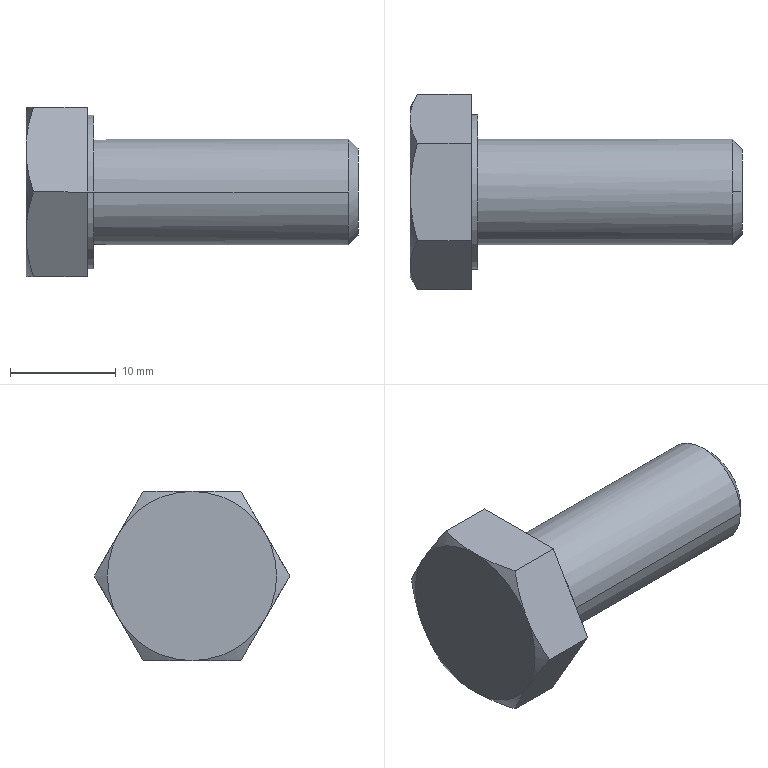Part | SolidWorks | features BaseBody 1 | 1 solid | 22 faces | box 31.4 x 18.475 x 16 mm | volume 3333 mm3 | plane 10 | cone 8 | cylinder 4 | commonest cylinder face diameters 10 x2 14.6 x2
STEP:
#1=CARTESIAN_POINT('',(0.,5.,0.));
#2=VERTEX_POINT('',#1);
#3=CARTESIAN_POINT('',(0.,-5.,0.));
#4=VERTEX_POINT('',#3);
#5=CARTESIAN_POINT('',(0.,0.,0.));
#6=DIRECTION('',(1.,0.,0.));
#7=DIRECTION('',(0.,1.,0.));
#8=AXIS2_PLACEMENT_3D('',#5,#6,#7);
#9=CIRCLE('',#8,5.);
#10=EDGE_CURVE('',#2,#4,#9,.T.);
#11=ORIENTED_EDGE('',*,*,#10,.T.);
#12=CARTESIAN_POINT('',(24.08,-5.,0.));
#13=VERTEX_POINT('',#12);
#14=CARTESIAN_POINT('',(13.25,-5.,0.));
#15=DIRECTION('',(1.,0.,0.));
#16=VECTOR('',#15,1000.);
#17=LINE('',#14,#16);
#18=EDGE_CURVE('',#4,#13,#17,.T.);
#19=ORIENTED_EDGE('',*,*,#18,.T.);
#20=CARTESIAN_POINT('',(24.08,0.,5.));
#21=VERTEX_POINT('',#20);
#22=CARTESIAN_POINT('',(24.08,0.,0.));
#23=DIRECTION('',(-1.,0.,0.));
#24=DIRECTION('',(0.,1.,0.));
#25=AXIS2_PLACEMENT_3D('',#22,#23,#24);
#26=CIRCLE('',#25,5.);
#27=EDGE_CURVE('',#13,#21,#26,.T.);
#28=ORIENTED_EDGE('',*,*,#27,.T.);
#29=CARTESIAN_POINT('',(24.08,5.,0.));
#30=VERTEX_POINT('',#29);
#31=CARTESIAN_POINT('',(24.08,0.,0.));
#32=DIRECTION('',(-1.,0.,0.));
#33=DIRECTION('',(0.,1.,0.));
#34=AXIS2_PLACEMENT_3D('',#31,#32,#33);
#35=CIRCLE('',#34,5.);
#36=EDGE_CURVE('',#21,#30,#35,.T.);
#37=ORIENTED_EDGE('',*,*,#36,.T.);
#38=CARTESIAN_POINT('',(13.25,5.,0.));
#39=DIRECTION('',(1.,0.,0.));
#40=VECTOR('',#39,1000.);
#41=LINE('',#38,#40);
#42=EDGE_CURVE('',#2,#30,#41,.T.);
#43=ORIENTED_EDGE('',*,*,#42,.F.);
#44=EDGE_LOOP('',(#11,#19,#28,#37,#43));
#45=FACE_OUTER_BOUND('',#44,.T.);
#46=CARTESIAN_POINT('',(13.25,0.,0.));
#47=DIRECTION('',(1.,0.,0.));
#48=DIRECTION('',(0.,1.,0.));
#49=AXIS2_PLACEMENT_3D('',#46,#47,#48);
#50=CYLINDRICAL_SURFACE('',#49,5.);
#51=ADVANCED_FACE('',(#45),#50,.T.);
#52=CARTESIAN_POINT('',(25.,0.,4.08));
#53=VERTEX_POINT('',#52);
#54=CARTESIAN_POINT('',(25.,0.,-4.08));
#55=VERTEX_POINT('',#54);
#56=CARTESIAN_POINT('',(25.,0.,0.));
#57=DIRECTION('',(-1.,0.,0.));
#58=DIRECTION('',(0.,0.,1.));
#59=AXIS2_PLACEMENT_3D('',#56,#57,#58);
#60=CIRCLE('',#59,4.08);
#61=EDGE_CURVE('',#53,#55,#60,.T.);
#62=ORIENTED_EDGE('',*,*,#61,.T.);
#63=CARTESIAN_POINT('',(24.08,0.,-5.));
#64=VERTEX_POINT('',#63);
#65=CARTESIAN_POINT('',(24.08,0.,-5.));
#66=DIRECTION('',(-0.7071,0.,-0.7071));
#67=VECTOR('',#66,1000.);
#68=LINE('',#65,#67);
#69=EDGE_CURVE('',#55,#64,#68,.T.);
#70=ORIENTED_EDGE('',*,*,#69,.T.);
#71=CARTESIAN_POINT('',(24.08,0.,0.));
#72=DIRECTION('',(-1.,0.,0.));
#73=DIRECTION('',(0.,1.,0.));
#74=AXIS2_PLACEMENT_3D('',#71,#72,#73);
#75=CIRCLE('',#74,5.);
#76=EDGE_CURVE('',#30,#64,#75,.T.);
#77=ORIENTED_EDGE('',*,*,#76,.F.);
#78=ORIENTED_EDGE('',*,*,#36,.F.);
#79=CARTESIAN_POINT('',(24.08,0.,5.));
#80=DIRECTION('',(-0.7071,0.,0.7071));
#81=VECTOR('',#80,1000.);
#82=LINE('',#79,#81);
#83=EDGE_CURVE('',#53,#21,#82,.T.);
#84=ORIENTED_EDGE('',*,*,#83,.F.);
#85=EDGE_LOOP('',(#62,#70,#77,#78,#84));
#86=FACE_OUTER_BOUND('',#85,.T.);
#87=CARTESIAN_POINT('',(24.08,0.,0.));
#88=DIRECTION('',(-1.,0.,0.));
#89=DIRECTION('',(0.,0.,1.));
#90=AXIS2_PLACEMENT_3D('',#87,#88,#89);
#91=CONICAL_SURFACE('',#90,5.,0.7853);
#92=ADVANCED_FACE('',(#86),#91,.T.);
#93=CARTESIAN_POINT('',(-0.6001,7.3,0.));
#94=VERTEX_POINT('',#93);
#95=CARTESIAN_POINT('',(-0.6001,-7.3,0.));
#96=VERTEX_POINT('',#95);
#97=CARTESIAN_POINT('',(-0.6001,0.,0.));
#98=DIRECTION('',(1.,0.,0.));
#99=DIRECTION('',(0.,1.,0.));
#100=AXIS2_PLACEMENT_3D('',#97,#98,#99);
#101=CIRCLE('',#100,7.3);
#102=EDGE_CURVE('',#94,#96,#101,.T.);
#103=ORIENTED_EDGE('',*,*,#102,.T.);
#104=CARTESIAN_POINT('',(0.,-7.3,0.));
#105=VERTEX_POINT('',#104);
#106=CARTESIAN_POINT('',(-0.3,-7.3,0.));
#107=DIRECTION('',(1.,0.,0.));
#108=VECTOR('',#107,1000.);
#109=LINE('',#106,#108);
#110=EDGE_CURVE('',#96,#105,#109,.T.);
#111=ORIENTED_EDGE('',*,*,#110,.T.);
#112=CARTESIAN_POINT('',(0.,7.3,0.));
#113=VERTEX_POINT('',#112);
#114=CARTESIAN_POINT('',(0.,0.,0.));
#115=DIRECTION('',(1.,0.,0.));
#116=DIRECTION('',(0.,1.,0.));
#117=AXIS2_PLACEMENT_3D('',#114,#115,#116);
#118=CIRCLE('',#117,7.3);
#119=EDGE_CURVE('',#113,#105,#118,.T.);
#120=ORIENTED_EDGE('',*,*,#119,.F.);
#121=CARTESIAN_POINT('',(-0.3,7.3,0.));
#122=DIRECTION('',(1.,0.,0.));
#123=VECTOR('',#122,1000.);
#124=LINE('',#121,#123);
#125=EDGE_CURVE('',#94,#113,#124,.T.);
#126=ORIENTED_EDGE('',*,*,#125,.F.);
#127=EDGE_LOOP('',(#103,#111,#120,#126));
#128=FACE_OUTER_BOUND('',#127,.T.);
#129=CARTESIAN_POINT('',(-0.3,0.,0.));
#130=DIRECTION('',(1.,0.,0.));
#131=DIRECTION('',(0.,1.,0.));
#132=AXIS2_PLACEMENT_3D('',#129,#130,#131);
#133=CYLINDRICAL_SURFACE('',#132,7.3);
#134=ADVANCED_FACE('',(#128),#133,.T.);
#135=ORIENTED_EDGE('',*,*,#18,.F.);
#136=CARTESIAN_POINT('',(0.,0.,0.));
#137=DIRECTION('',(1.,0.,0.));
#138=DIRECTION('',(0.,1.,0.));
#139=AXIS2_PLACEMENT_3D('',#136,#137,#138);
#140=CIRCLE('',#139,5.);
#141=EDGE_CURVE('',#4,#2,#140,.T.);
#142=ORIENTED_EDGE('',*,*,#141,.T.);
#143=ORIENTED_EDGE('',*,*,#42,.T.);
#144=ORIENTED_EDGE('',*,*,#76,.T.);
#145=CARTESIAN_POINT('',(24.08,0.,0.));
#146=DIRECTION('',(-1.,0.,0.));
#147=DIRECTION('',(0.,1.,0.));
#148=AXIS2_PLACEMENT_3D('',#145,#146,#147);
#149=CIRCLE('',#148,5.);
#150=EDGE_CURVE('',#64,#13,#149,.T.);
#151=ORIENTED_EDGE('',*,*,#150,.T.);
#152=EDGE_LOOP('',(#135,#142,#143,#144,#151));
#153=FACE_OUTER_BOUND('',#152,.T.);
#154=CARTESIAN_POINT('',(13.25,0.,0.));
#155=DIRECTION('',(1.,0.,0.));
#156=DIRECTION('',(0.,1.,0.));
#157=AXIS2_PLACEMENT_3D('',#154,#155,#156);
#158=CYLINDRICAL_SURFACE('',#157,5.);
#159=ADVANCED_FACE('',(#153),#158,.T.);
#160=ORIENTED_EDGE('',*,*,#69,.F.);
#161=CARTESIAN_POINT('',(25.,0.,0.));
#162=DIRECTION('',(-1.,0.,0.));
#163=DIRECTION('',(0.,0.,1.));
#164=AXIS2_PLACEMENT_3D('',#161,#162,#163);
#165=CIRCLE('',#164,4.08);
#166=EDGE_CURVE('',#55,#53,#165,.T.);
#167=ORIENTED_EDGE('',*,*,#166,.T.);
#168=ORIENTED_EDGE('',*,*,#83,.T.);
#169=ORIENTED_EDGE('',*,*,#27,.F.);
#170=ORIENTED_EDGE('',*,*,#150,.F.);
#171=EDGE_LOOP('',(#160,#167,#168,#169,#170));
#172=FACE_OUTER_BOUND('',#171,.T.);
#173=CARTESIAN_POINT('',(24.08,0.,0.));
#174=DIRECTION('',(-1.,0.,0.));
#175=DIRECTION('',(0.,0.,1.));
#176=AXIS2_PLACEMENT_3D('',#173,#174,#175);
#177=CONICAL_SURFACE('',#176,5.,0.7853);
#178=ADVANCED_FACE('',(#172),#177,.T.);
#179=ORIENTED_EDGE('',*,*,#10,.F.);
#180=ORIENTED_EDGE('',*,*,#141,.F.);
#181=EDGE_LOOP('',(#179,#180));
#182=FACE_BOUND('',#181,.T.);
#183=ORIENTED_EDGE('',*,*,#119,.T.);
#184=CARTESIAN_POINT('',(0.,0.,0.));
#185=DIRECTION('',(1.,0.,0.));
#186=DIRECTION('',(0.,1.,0.));
#187=AXIS2_PLACEMENT_3D('',#184,#185,#186);
#188=CIRCLE('',#187,7.3);
#189=EDGE_CURVE('',#105,#113,#188,.T.);
#190=ORIENTED_EDGE('',*,*,#189,.T.);
#191=EDGE_LOOP('',(#183,#190));
#192=FACE_OUTER_BOUND('',#191,.T.);
#193=CARTESIAN_POINT('',(0.,6.15,0.));
#194=DIRECTION('',(1.,0.,0.));
#195=DIRECTION('',(0.,1.,0.));
#196=AXIS2_PLACEMENT_3D('',#193,#194,#195);
#197=PLANE('',#196);
#198=ADVANCED_FACE('',(#182,#192),#197,.T.);
#199=ORIENTED_EDGE('',*,*,#61,.F.);
#200=ORIENTED_EDGE('',*,*,#166,.F.);
#201=EDGE_LOOP('',(#199,#200));
#202=FACE_OUTER_BOUND('',#201,.T.);
#203=CARTESIAN_POINT('',(25.,2.5,0.));
#204=DIRECTION('',(1.,0.,0.));
#205=DIRECTION('',(0.,1.,0.));
#206=AXIS2_PLACEMENT_3D('',#203,#204,#205);
#207=PLANE('',#206);
#208=ADVANCED_FACE('',(#202),#207,.T.);
#209=ORIENTED_EDGE('',*,*,#110,.F.);
#210=CARTESIAN_POINT('',(-0.6001,0.,0.));
#211=DIRECTION('',(1.,0.,0.));
#212=DIRECTION('',(0.,1.,0.));
#213=AXIS2_PLACEMENT_3D('',#210,#211,#212);
#214=CIRCLE('',#213,7.3);
#215=EDGE_CURVE('',#96,#94,#214,.T.);
#216=ORIENTED_EDGE('',*,*,#215,.T.);
#217=ORIENTED_EDGE('',*,*,#125,.T.);
#218=ORIENTED_EDGE('',*,*,#189,.F.);
#219=EDGE_LOOP('',(#209,#216,#217,#218));
#220=FACE_OUTER_BOUND('',#219,.T.);
#221=CARTESIAN_POINT('',(-0.3,0.,0.));
#222=DIRECTION('',(1.,0.,0.));
#223=DIRECTION('',(0.,1.,0.));
#224=AXIS2_PLACEMENT_3D('',#221,#222,#223);
#225=CYLINDRICAL_SURFACE('',#224,7.3);
#226=ADVANCED_FACE('',(#220),#225,.T.);
#227=ORIENTED_EDGE('',*,*,#102,.F.);
#228=ORIENTED_EDGE('',*,*,#215,.F.);
#229=EDGE_LOOP('',(#227,#228));
#230=FACE_BOUND('',#229,.T.);
#231=CARTESIAN_POINT('',(-0.6001,-4.619,-8.));
#232=VERTEX_POINT('',#231);
#233=CARTESIAN_POINT('',(-0.6001,4.619,-8.));
#234=VERTEX_POINT('',#233);
#235=CARTESIAN_POINT('',(-0.6001,0.,-8.));
#236=DIRECTION('',(0.,1.,0.));
#237=VECTOR('',#236,1000.);
#238=LINE('',#235,#237);
#239=EDGE_CURVE('',#232,#234,#238,.T.);
#240=ORIENTED_EDGE('',*,*,#239,.T.);
#241=CARTESIAN_POINT('',(-0.6001,9.238,0.));
#242=VERTEX_POINT('',#241);
#243=CARTESIAN_POINT('',(-0.6001,4.619,-8.));
#244=DIRECTION('',(0.,0.5,0.866));
#245=VECTOR('',#244,1000.);
#246=LINE('',#243,#245);
#247=EDGE_CURVE('',#234,#242,#246,.T.);
#248=ORIENTED_EDGE('',*,*,#247,.T.);
#249=CARTESIAN_POINT('',(-0.6001,4.619,8.));
#250=VERTEX_POINT('',#249);
#251=CARTESIAN_POINT('',(-0.6001,9.238,0.));
#252=DIRECTION('',(0.,-0.5,0.866));
#253=VECTOR('',#252,1000.);
#254=LINE('',#251,#253);
#255=EDGE_CURVE('',#242,#250,#254,.T.);
#256=ORIENTED_EDGE('',*,*,#255,.T.);
#257=CARTESIAN_POINT('',(-0.6001,-4.619,8.));
#258=VERTEX_POINT('',#257);
#259=CARTESIAN_POINT('',(-0.6001,0.,8.));
#260=DIRECTION('',(0.,-1.,0.));
#261=VECTOR('',#260,1000.);
#262=LINE('',#259,#261);
#263=EDGE_CURVE('',#250,#258,#262,.T.);
#264=ORIENTED_EDGE('',*,*,#263,.T.);
#265=CARTESIAN_POINT('',(-0.6001,-9.238,0.));
#266=VERTEX_POINT('',#265);
#267=CARTESIAN_POINT('',(-0.6001,-4.619,8.));
#268=DIRECTION('',(0.,-0.5,-0.866));
#269=VECTOR('',#268,1000.);
#270=LINE('',#267,#269);
#271=EDGE_CURVE('',#258,#266,#270,.T.);
#272=ORIENTED_EDGE('',*,*,#271,.T.);
#273=CARTESIAN_POINT('',(-0.6001,-9.238,0.));
#274=DIRECTION('',(0.,0.5,-0.866));
#275=VECTOR('',#274,1000.);
#276=LINE('',#273,#275);
#277=EDGE_CURVE('',#266,#232,#276,.T.);
#278=ORIENTED_EDGE('',*,*,#277,.T.);
#279=EDGE_LOOP('',(#240,#248,#256,#264,#272,#278));
#280=FACE_OUTER_BOUND('',#279,.T.);
#281=CARTESIAN_POINT('',(-0.6001,0.,0.));
#282=DIRECTION('',(1.,0.,0.));
#283=DIRECTION('',(0.,1.,0.));
#284=AXIS2_PLACEMENT_3D('',#281,#282,#283);
#285=PLANE('',#284);
#286=ADVANCED_FACE('',(#230,#280),#285,.T.);
#287=ORIENTED_EDGE('',*,*,#247,.F.);
#288=CARTESIAN_POINT('',(-5.686,4.619,-8.));
#289=VERTEX_POINT('',#288);
#290=CARTESIAN_POINT('',(-0.6001,4.619,-8.));
#291=DIRECTION('',(-1.,0.,0.));
#292=VECTOR('',#291,1000.);
#293=LINE('',#290,#292);
#294=EDGE_CURVE('',#234,#289,#293,.T.);
#295=ORIENTED_EDGE('',*,*,#294,.T.);
#296=CARTESIAN_POINT('',(-6.4,6.928,-4.));
#297=VERTEX_POINT('',#296);
#298=CARTESIAN_POINT('',(-5.686,4.619,-8.));
#299=CARTESIAN_POINT('',(-5.903,4.996,-7.347));
#300=CARTESIAN_POINT('',(-6.083,5.376,-6.688));
#301=CARTESIAN_POINT('',(-6.332,6.145,-5.356));
#302=CARTESIAN_POINT('',(-6.4,6.534,-4.683));
#303=CARTESIAN_POINT('',(-6.4,6.928,-4.));
#304=B_SPLINE_CURVE_WITH_KNOTS('',3,(#298,#299,#300,#301,#302,#303),.UNSPECIFIED.,.F.,.F.,(4,2,4),(0.,0.002337,0.004674),.UNSPECIFIED.);
#305=EDGE_CURVE('',#289,#297,#304,.T.);
#306=ORIENTED_EDGE('',*,*,#305,.T.);
#307=CARTESIAN_POINT('',(-5.686,9.238,0.));
#308=VERTEX_POINT('',#307);
#309=CARTESIAN_POINT('',(-6.4,6.928,-4.));
#310=CARTESIAN_POINT('',(-6.4,7.322,-3.317));
#311=CARTESIAN_POINT('',(-6.332,7.711,-2.644));
#312=CARTESIAN_POINT('',(-6.083,8.48,-1.312));
#313=CARTESIAN_POINT('',(-5.903,8.86,-0.6534));
#314=CARTESIAN_POINT('',(-5.686,9.238,0.));
#315=B_SPLINE_CURVE_WITH_KNOTS('',3,(#309,#310,#311,#312,#313,#314),.UNSPECIFIED.,.F.,.F.,(4,2,4),(0.,0.002337,0.004674),.UNSPECIFIED.);
#316=EDGE_CURVE('',#297,#308,#315,.T.);
#317=ORIENTED_EDGE('',*,*,#316,.T.);
#318=CARTESIAN_POINT('',(-0.6001,9.238,0.));
#319=DIRECTION('',(1.,0.,0.));
#320=VECTOR('',#319,1000.);
#321=LINE('',#318,#320);
#322=EDGE_CURVE('',#308,#242,#321,.T.);
#323=ORIENTED_EDGE('',*,*,#322,.T.);
#324=EDGE_LOOP('',(#287,#295,#306,#317,#323));
#325=FACE_OUTER_BOUND('',#324,.T.);
#326=CARTESIAN_POINT('',(-0.6001,4.619,-8.));
#327=DIRECTION('',(0.,0.866,-0.5));
#328=DIRECTION('',(0.,0.5,0.866));
#329=AXIS2_PLACEMENT_3D('',#326,#327,#328);
#330=PLANE('',#329);
#331=ADVANCED_FACE('',(#325),#330,.T.);
#332=ORIENTED_EDGE('',*,*,#239,.F.);
#333=CARTESIAN_POINT('',(-5.686,-4.619,-8.));
#334=VERTEX_POINT('',#333);
#335=CARTESIAN_POINT('',(-0.6001,-4.619,-8.));
#336=DIRECTION('',(-1.,0.,0.));
#337=VECTOR('',#336,1000.);
#338=LINE('',#335,#337);
#339=EDGE_CURVE('',#232,#334,#338,.T.);
#340=ORIENTED_EDGE('',*,*,#339,.T.);
#341=CARTESIAN_POINT('',(-6.4,0.,-8.));
#342=VERTEX_POINT('',#341);
#343=CARTESIAN_POINT('',(-5.686,-4.619,-8.));
#344=CARTESIAN_POINT('',(-5.903,-3.864,-8.));
#345=CARTESIAN_POINT('',(-6.083,-3.104,-8.));
#346=CARTESIAN_POINT('',(-6.332,-1.566,-8.));
#347=CARTESIAN_POINT('',(-6.4,-0.7882,-8.));
#348=CARTESIAN_POINT('',(-6.4,0.,-8.));
#349=B_SPLINE_CURVE_WITH_KNOTS('',3,(#343,#344,#345,#346,#347,#348),.UNSPECIFIED.,.F.,.F.,(4,2,4),(0.,0.002337,0.004674),.UNSPECIFIED.);
#350=EDGE_CURVE('',#334,#342,#349,.T.);
#351=ORIENTED_EDGE('',*,*,#350,.T.);
#352=CARTESIAN_POINT('',(-6.4,0.,-8.));
#353=CARTESIAN_POINT('',(-6.4,0.7882,-8.));
#354=CARTESIAN_POINT('',(-6.332,1.566,-8.));
#355=CARTESIAN_POINT('',(-6.083,3.104,-8.));
#356=CARTESIAN_POINT('',(-5.903,3.864,-8.));
#357=CARTESIAN_POINT('',(-5.686,4.619,-8.));
#358=B_SPLINE_CURVE_WITH_KNOTS('',3,(#352,#353,#354,#355,#356,#357),.UNSPECIFIED.,.F.,.F.,(4,2,4),(0.,0.002337,0.004674),.UNSPECIFIED.);
#359=EDGE_CURVE('',#342,#289,#358,.T.);
#360=ORIENTED_EDGE('',*,*,#359,.T.);
#361=ORIENTED_EDGE('',*,*,#294,.F.);
#362=EDGE_LOOP('',(#332,#340,#351,#360,#361));
#363=FACE_OUTER_BOUND('',#362,.T.);
#364=CARTESIAN_POINT('',(-0.6001,-4.619,-8.));
#365=DIRECTION('',(0.,0.,-1.));
#366=DIRECTION('',(0.,1.,0.));
#367=AXIS2_PLACEMENT_3D('',#364,#365,#366);
#368=PLANE('',#367);
#369=ADVANCED_FACE('',(#363),#368,.T.);
#370=CARTESIAN_POINT('',(-5.686,-9.238,0.));
#371=VERTEX_POINT('',#370);
#372=CARTESIAN_POINT('',(-0.6001,-9.238,0.));
#373=DIRECTION('',(-1.,0.,0.));
#374=VECTOR('',#373,1000.);
#375=LINE('',#372,#374);
#376=EDGE_CURVE('',#266,#371,#375,.T.);
#377=ORIENTED_EDGE('',*,*,#376,.T.);
#378=CARTESIAN_POINT('',(-6.4,-6.928,-4.));
#379=VERTEX_POINT('',#378);
#380=CARTESIAN_POINT('',(-5.686,-9.238,0.));
#381=CARTESIAN_POINT('',(-5.903,-8.86,-0.6534));
#382=CARTESIAN_POINT('',(-6.083,-8.48,-1.312));
#383=CARTESIAN_POINT('',(-6.332,-7.711,-2.644));
#384=CARTESIAN_POINT('',(-6.4,-7.322,-3.317));
#385=CARTESIAN_POINT('',(-6.4,-6.928,-4.));
#386=B_SPLINE_CURVE_WITH_KNOTS('',3,(#380,#381,#382,#383,#384,#385),.UNSPECIFIED.,.F.,.F.,(4,2,4),(0.,0.002337,0.004674),.UNSPECIFIED.);
#387=EDGE_CURVE('',#371,#379,#386,.T.);
#388=ORIENTED_EDGE('',*,*,#387,.T.);
#389=CARTESIAN_POINT('',(-6.4,-6.928,-4.));
#390=CARTESIAN_POINT('',(-6.4,-6.534,-4.683));
#391=CARTESIAN_POINT('',(-6.332,-6.145,-5.356));
#392=CARTESIAN_POINT('',(-6.083,-5.376,-6.688));
#393=CARTESIAN_POINT('',(-5.903,-4.996,-7.347));
#394=CARTESIAN_POINT('',(-5.686,-4.619,-8.));
#395=B_SPLINE_CURVE_WITH_KNOTS('',3,(#389,#390,#391,#392,#393,#394),.UNSPECIFIED.,.F.,.F.,(4,2,4),(0.,0.002337,0.004674),.UNSPECIFIED.);
#396=EDGE_CURVE('',#379,#334,#395,.T.);
#397=ORIENTED_EDGE('',*,*,#396,.T.);
#398=ORIENTED_EDGE('',*,*,#339,.F.);
#399=ORIENTED_EDGE('',*,*,#277,.F.);
#400=EDGE_LOOP('',(#377,#388,#397,#398,#399));
#401=FACE_OUTER_BOUND('',#400,.T.);
#402=CARTESIAN_POINT('',(-0.6001,-9.238,0.));
#403=DIRECTION('',(0.,-0.866,-0.5));
#404=DIRECTION('',(0.,0.5,-0.866));
#405=AXIS2_PLACEMENT_3D('',#402,#403,#404);
#406=PLANE('',#405);
#407=ADVANCED_FACE('',(#401),#406,.T.);
#408=CARTESIAN_POINT('',(-5.686,-4.619,8.));
#409=VERTEX_POINT('',#408);
#410=CARTESIAN_POINT('',(-0.6001,-4.619,8.));
#411=DIRECTION('',(-1.,0.,0.));
#412=VECTOR('',#411,1000.);
#413=LINE('',#410,#412);
#414=EDGE_CURVE('',#258,#409,#413,.T.);
#415=ORIENTED_EDGE('',*,*,#414,.T.);
#416=CARTESIAN_POINT('',(-6.4,-6.928,4.));
#417=VERTEX_POINT('',#416);
#418=CARTESIAN_POINT('',(-5.686,-4.619,8.));
#419=CARTESIAN_POINT('',(-5.903,-4.996,7.347));
#420=CARTESIAN_POINT('',(-6.083,-5.376,6.688));
#421=CARTESIAN_POINT('',(-6.332,-6.145,5.356));
#422=CARTESIAN_POINT('',(-6.4,-6.534,4.683));
#423=CARTESIAN_POINT('',(-6.4,-6.928,4.));
#424=B_SPLINE_CURVE_WITH_KNOTS('',3,(#418,#419,#420,#421,#422,#423),.UNSPECIFIED.,.F.,.F.,(4,2,4),(0.,0.002337,0.004674),.UNSPECIFIED.);
#425=EDGE_CURVE('',#409,#417,#424,.T.);
#426=ORIENTED_EDGE('',*,*,#425,.T.);
#427=CARTESIAN_POINT('',(-6.4,-6.928,4.));
#428=CARTESIAN_POINT('',(-6.4,-7.322,3.317));
#429=CARTESIAN_POINT('',(-6.332,-7.711,2.644));
#430=CARTESIAN_POINT('',(-6.083,-8.48,1.312));
#431=CARTESIAN_POINT('',(-5.903,-8.86,0.6534));
#432=CARTESIAN_POINT('',(-5.686,-9.238,0.));
#433=B_SPLINE_CURVE_WITH_KNOTS('',3,(#427,#428,#429,#430,#431,#432),.UNSPECIFIED.,.F.,.F.,(4,2,4),(0.,0.002337,0.004674),.UNSPECIFIED.);
#434=EDGE_CURVE('',#417,#371,#433,.T.);
#435=ORIENTED_EDGE('',*,*,#434,.T.);
#436=ORIENTED_EDGE('',*,*,#376,.F.);
#437=ORIENTED_EDGE('',*,*,#271,.F.);
#438=EDGE_LOOP('',(#415,#426,#435,#436,#437));
#439=FACE_OUTER_BOUND('',#438,.T.);
#440=CARTESIAN_POINT('',(-0.6001,-4.619,8.));
#441=DIRECTION('',(0.,-0.866,0.5));
#442=DIRECTION('',(0.,-0.5,-0.866));
#443=AXIS2_PLACEMENT_3D('',#440,#441,#442);
#444=PLANE('',#443);
#445=ADVANCED_FACE('',(#439),#444,.T.);
#446=CARTESIAN_POINT('',(-5.686,4.619,8.));
#447=VERTEX_POINT('',#446);
#448=CARTESIAN_POINT('',(-0.6001,4.619,8.));
#449=DIRECTION('',(-1.,0.,0.));
#450=VECTOR('',#449,1000.);
#451=LINE('',#448,#450);
#452=EDGE_CURVE('',#250,#447,#451,.T.);
#453=ORIENTED_EDGE('',*,*,#452,.T.);
#454=CARTESIAN_POINT('',(-6.4,0.,8.));
#455=VERTEX_POINT('',#454);
#456=CARTESIAN_POINT('',(-5.686,4.619,8.));
#457=CARTESIAN_POINT('',(-5.903,3.864,8.));
#458=CARTESIAN_POINT('',(-6.083,3.104,8.));
#459=CARTESIAN_POINT('',(-6.332,1.566,8.));
#460=CARTESIAN_POINT('',(-6.4,0.7882,8.));
#461=CARTESIAN_POINT('',(-6.4,0.,8.));
#462=B_SPLINE_CURVE_WITH_KNOTS('',3,(#456,#457,#458,#459,#460,#461),.UNSPECIFIED.,.F.,.F.,(4,2,4),(0.,0.002337,0.004674),.UNSPECIFIED.);
#463=EDGE_CURVE('',#447,#455,#462,.T.);
#464=ORIENTED_EDGE('',*,*,#463,.T.);
#465=CARTESIAN_POINT('',(-6.4,0.,8.));
#466=CARTESIAN_POINT('',(-6.4,-0.7882,8.));
#467=CARTESIAN_POINT('',(-6.332,-1.566,8.));
#468=CARTESIAN_POINT('',(-6.083,-3.104,8.));
#469=CARTESIAN_POINT('',(-5.903,-3.864,8.));
#470=CARTESIAN_POINT('',(-5.686,-4.619,8.));
#471=B_SPLINE_CURVE_WITH_KNOTS('',3,(#465,#466,#467,#468,#469,#470),.UNSPECIFIED.,.F.,.F.,(4,2,4),(0.,0.002337,0.004674),.UNSPECIFIED.);
#472=EDGE_CURVE('',#455,#409,#471,.T.);
#473=ORIENTED_EDGE('',*,*,#472,.T.);
#474=ORIENTED_EDGE('',*,*,#414,.F.);
#475=ORIENTED_EDGE('',*,*,#263,.F.);
#476=EDGE_LOOP('',(#453,#464,#473,#474,#475));
#477=FACE_OUTER_BOUND('',#476,.T.);
#478=CARTESIAN_POINT('',(-0.6001,4.619,8.));
#479=DIRECTION('',(0.,0.,1.));
#480=DIRECTION('',(0.,-1.,0.));
#481=AXIS2_PLACEMENT_3D('',#478,#479,#480);
#482=PLANE('',#481);
#483=ADVANCED_FACE('',(#477),#482,.T.);
#484=ORIENTED_EDGE('',*,*,#255,.F.);
#485=ORIENTED_EDGE('',*,*,#322,.F.);
#486=CARTESIAN_POINT('',(-6.4,6.928,4.));
#487=VERTEX_POINT('',#486);
#488=CARTESIAN_POINT('',(-5.686,9.238,0.));
#489=CARTESIAN_POINT('',(-5.903,8.86,0.6534));
#490=CARTESIAN_POINT('',(-6.083,8.48,1.312));
#491=CARTESIAN_POINT('',(-6.332,7.711,2.644));
#492=CARTESIAN_POINT('',(-6.4,7.322,3.317));
#493=CARTESIAN_POINT('',(-6.4,6.928,4.));
#494=B_SPLINE_CURVE_WITH_KNOTS('',3,(#488,#489,#490,#491,#492,#493),.UNSPECIFIED.,.F.,.F.,(4,2,4),(0.,0.002337,0.004674),.UNSPECIFIED.);
#495=EDGE_CURVE('',#308,#487,#494,.T.);
#496=ORIENTED_EDGE('',*,*,#495,.T.);
#497=CARTESIAN_POINT('',(-6.4,6.928,4.));
#498=CARTESIAN_POINT('',(-6.4,6.534,4.683));
#499=CARTESIAN_POINT('',(-6.332,6.145,5.356));
#500=CARTESIAN_POINT('',(-6.083,5.376,6.688));
#501=CARTESIAN_POINT('',(-5.903,4.996,7.347));
#502=CARTESIAN_POINT('',(-5.686,4.619,8.));
#503=B_SPLINE_CURVE_WITH_KNOTS('',3,(#497,#498,#499,#500,#501,#502),.UNSPECIFIED.,.F.,.F.,(4,2,4),(0.,0.002337,0.004674),.UNSPECIFIED.);
#504=EDGE_CURVE('',#487,#447,#503,.T.);
#505=ORIENTED_EDGE('',*,*,#504,.T.);
#506=ORIENTED_EDGE('',*,*,#452,.F.);
#507=EDGE_LOOP('',(#484,#485,#496,#505,#506));
#508=FACE_OUTER_BOUND('',#507,.T.);
#509=CARTESIAN_POINT('',(-0.6001,9.238,0.));
#510=DIRECTION('',(0.,0.866,0.5));
#511=DIRECTION('',(0.,-0.5,0.866));
#512=AXIS2_PLACEMENT_3D('',#509,#510,#511);
#513=PLANE('',#512);
#514=ADVANCED_FACE('',(#508),#513,.T.);
#515=CARTESIAN_POINT('',(-6.4,0.,0.));
#516=DIRECTION('',(1.,0.,0.));
#517=DIRECTION('',(0.,0.,-1.));
#518=AXIS2_PLACEMENT_3D('',#515,#516,#517);
#519=CIRCLE('',#518,8.);
#520=EDGE_CURVE('',#297,#487,#519,.T.);
#521=ORIENTED_EDGE('',*,*,#520,.T.);
#522=ORIENTED_EDGE('',*,*,#495,.F.);
#523=ORIENTED_EDGE('',*,*,#316,.F.);
#524=EDGE_LOOP('',(#521,#522,#523));
#525=FACE_OUTER_BOUND('',#524,.T.);
#526=CARTESIAN_POINT('',(-5.681,0.,0.));
#527=DIRECTION('',(1.,0.,0.));
#528=DIRECTION('',(0.,0.,-1.));
#529=AXIS2_PLACEMENT_3D('',#526,#527,#528);
#530=CONICAL_SURFACE('',#529,9.245,1.047);
#531=ADVANCED_FACE('',(#525),#530,.T.);
#532=CARTESIAN_POINT('',(-6.4,0.,0.));
#533=DIRECTION('',(1.,0.,0.));
#534=DIRECTION('',(0.,0.,-1.));
#535=AXIS2_PLACEMENT_3D('',#532,#533,#534);
#536=CIRCLE('',#535,8.);
#537=EDGE_CURVE('',#342,#297,#536,.T.);
#538=ORIENTED_EDGE('',*,*,#537,.T.);
#539=ORIENTED_EDGE('',*,*,#305,.F.);
#540=ORIENTED_EDGE('',*,*,#359,.F.);
#541=EDGE_LOOP('',(#538,#539,#540));
#542=FACE_OUTER_BOUND('',#541,.T.);
#543=CARTESIAN_POINT('',(-5.681,0.,0.));
#544=DIRECTION('',(1.,0.,0.));
#545=DIRECTION('',(0.,0.,-1.));
#546=AXIS2_PLACEMENT_3D('',#543,#544,#545);
#547=CONICAL_SURFACE('',#546,9.245,1.047);
#548=ADVANCED_FACE('',(#542),#547,.T.);
#549=ORIENTED_EDGE('',*,*,#396,.F.);
#550=CARTESIAN_POINT('',(-6.4,0.,0.));
#551=DIRECTION('',(1.,0.,0.));
#552=DIRECTION('',(0.,0.,-1.));
#553=AXIS2_PLACEMENT_3D('',#550,#551,#552);
#554=CIRCLE('',#553,8.);
#555=EDGE_CURVE('',#379,#342,#554,.T.);
#556=ORIENTED_EDGE('',*,*,#555,.T.);
#557=ORIENTED_EDGE('',*,*,#350,.F.);
#558=EDGE_LOOP('',(#549,#556,#557));
#559=FACE_OUTER_BOUND('',#558,.T.);
#560=CARTESIAN_POINT('',(-5.681,0.,0.));
#561=DIRECTION('',(1.,0.,0.));
#562=DIRECTION('',(0.,0.,-1.));
#563=AXIS2_PLACEMENT_3D('',#560,#561,#562);
#564=CONICAL_SURFACE('',#563,9.245,1.047);
#565=ADVANCED_FACE('',(#559),#564,.T.);
#566=ORIENTED_EDGE('',*,*,#434,.F.);
#567=CARTESIAN_POINT('',(-6.4,0.,0.));
#568=DIRECTION('',(1.,0.,0.));
#569=DIRECTION('',(0.,0.,-1.));
#570=AXIS2_PLACEMENT_3D('',#567,#568,#569);
#571=CIRCLE('',#570,8.);
#572=EDGE_CURVE('',#417,#379,#571,.T.);
#573=ORIENTED_EDGE('',*,*,#572,.T.);
#574=ORIENTED_EDGE('',*,*,#387,.F.);
#575=EDGE_LOOP('',(#566,#573,#574));
#576=FACE_OUTER_BOUND('',#575,.T.);
#577=CARTESIAN_POINT('',(-5.681,0.,0.));
#578=DIRECTION('',(1.,0.,0.));
#579=DIRECTION('',(0.,0.,-1.));
#580=AXIS2_PLACEMENT_3D('',#577,#578,#579);
#581=CONICAL_SURFACE('',#580,9.245,1.047);
#582=ADVANCED_FACE('',(#576),#581,.T.);
#583=ORIENTED_EDGE('',*,*,#472,.F.);
#584=CARTESIAN_POINT('',(-6.4,0.,0.));
#585=DIRECTION('',(1.,0.,0.));
#586=DIRECTION('',(0.,0.,-1.));
#587=AXIS2_PLACEMENT_3D('',#584,#585,#586);
#588=CIRCLE('',#587,8.);
#589=EDGE_CURVE('',#455,#417,#588,.T.);
#590=ORIENTED_EDGE('',*,*,#589,.T.);
#591=ORIENTED_EDGE('',*,*,#425,.F.);
#592=EDGE_LOOP('',(#583,#590,#591));
#593=FACE_OUTER_BOUND('',#592,.T.);
#594=CARTESIAN_POINT('',(-5.681,0.,0.));
#595=DIRECTION('',(1.,0.,0.));
#596=DIRECTION('',(0.,0.,-1.));
#597=AXIS2_PLACEMENT_3D('',#594,#595,#596);
#598=CONICAL_SURFACE('',#597,9.245,1.047);
#599=ADVANCED_FACE('',(#593),#598,.T.);
#600=CARTESIAN_POINT('',(-6.4,0.,0.));
#601=DIRECTION('',(1.,0.,0.));
#602=DIRECTION('',(0.,0.,-1.));
#603=AXIS2_PLACEMENT_3D('',#600,#601,#602);
#604=CIRCLE('',#603,8.);
#605=EDGE_CURVE('',#487,#455,#604,.T.);
#606=ORIENTED_EDGE('',*,*,#605,.T.);
#607=ORIENTED_EDGE('',*,*,#463,.F.);
#608=ORIENTED_EDGE('',*,*,#504,.F.);
#609=EDGE_LOOP('',(#606,#607,#608));
#610=FACE_OUTER_BOUND('',#609,.T.);
#611=CARTESIAN_POINT('',(-5.681,0.,0.));
#612=DIRECTION('',(1.,0.,0.));
#613=DIRECTION('',(0.,0.,-1.));
#614=AXIS2_PLACEMENT_3D('',#611,#612,#613);
#615=CONICAL_SURFACE('',#614,9.245,1.047);
#616=ADVANCED_FACE('',(#610),#615,.T.);
#617=ORIENTED_EDGE('',*,*,#520,.F.);
#618=ORIENTED_EDGE('',*,*,#537,.F.);
#619=ORIENTED_EDGE('',*,*,#555,.F.);
#620=ORIENTED_EDGE('',*,*,#572,.F.);
#621=ORIENTED_EDGE('',*,*,#589,.F.);
#622=ORIENTED_EDGE('',*,*,#605,.F.);
#623=EDGE_LOOP('',(#617,#618,#619,#620,#621,#622));
#624=FACE_OUTER_BOUND('',#623,.T.);
#625=CARTESIAN_POINT('',(-6.4,0.,0.));
#626=DIRECTION('',(1.,0.,0.));
#627=DIRECTION('',(0.,1.,0.));
#628=AXIS2_PLACEMENT_3D('',#625,#626,#627);
#629=PLANE('',#628);
#630=ADVANCED_FACE('',(#624),#629,.F.);
#631=CLOSED_SHELL('',(#51,#92,#134,#159,#178,#198,#208,#226,#286,#331,#369,#407,#445,#483,#514,#531,#548,#565,#582,#599,#616,#630));
#632=MANIFOLD_SOLID_BREP('',#631);
#633=CARTESIAN_POINT('',(0.,0.,0.));
#634=DIRECTION('',(0.,0.,1.));
#635=DIRECTION('',(1.,0.,0.));
#636=AXIS2_PLACEMENT_3D('',#633,#634,#635);
#637=(LENGTH_UNIT()NAMED_UNIT(*)SI_UNIT(.MILLI.,.METRE.));
#638=UNCERTAINTY_MEASURE_WITH_UNIT(LENGTH_MEASURE(0.00001),#637,'','');
#639=(NAMED_UNIT(*)PLANE_ANGLE_UNIT()SI_UNIT($,.RADIAN.));
#640=(NAMED_UNIT(*)SI_UNIT($,.STERADIAN.)SOLID_ANGLE_UNIT());
#641=(GEOMETRIC_REPRESENTATION_CONTEXT(3)GLOBAL_UNCERTAINTY_ASSIGNED_CONTEXT((#638))GLOBAL_UNIT_ASSIGNED_CONTEXT((#637,#639,#640))REPRESENTATION_CONTEXT('',''));
#642=ADVANCED_BREP_SHAPE_REPRESENTATION('',(#632,#636),#641);